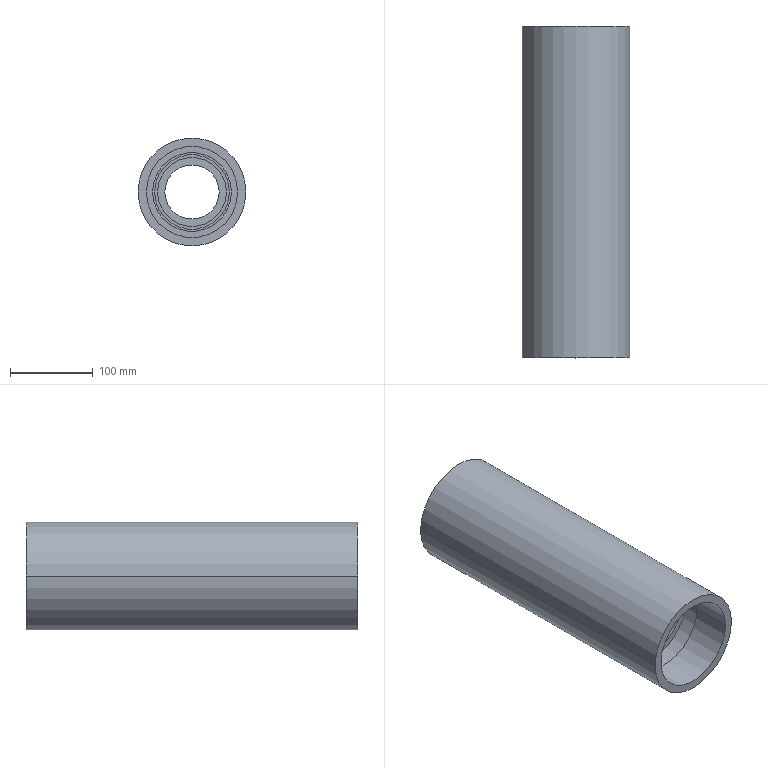Part | SolidWorks | features BaseBody 1 | 1 solid | 36 faces | box 130 x 400 x 130 mm | volume 2263150 mm3 | cylinder 24 | plane 12 | commonest cylinder face diameters 95 x6 110 x6 65.5 x2 76 x2 83 x2 90 x2
STEP:
#1=CARTESIAN_POINT('',(-2197.95,1104.894,-1577.624));
#2=VERTEX_POINT('',#1);
#3=CARTESIAN_POINT('',(-2197.95,704.894,-1577.624));
#4=VERTEX_POINT('',#3);
#5=CARTESIAN_POINT('',(-2197.95,1104.894,-1577.624));
#6=DIRECTION('',(0.,-1.,0.));
#7=VECTOR('',#6,1000.);
#8=LINE('',#5,#7);
#9=EDGE_CURVE('',#2,#4,#8,.T.);
#10=ORIENTED_EDGE('',*,*,#9,.F.);
#11=CARTESIAN_POINT('',(-2067.95,1104.894,-1577.624));
#12=VERTEX_POINT('',#11);
#13=CARTESIAN_POINT('',(-2132.95,1104.894,-1577.624));
#14=DIRECTION('',(0.,1.,0.));
#15=DIRECTION('',(1.,0.,0.));
#16=AXIS2_PLACEMENT_3D('',#13,#14,#15);
#17=CIRCLE('',#16,65.);
#18=EDGE_CURVE('',#12,#2,#17,.T.);
#19=ORIENTED_EDGE('',*,*,#18,.F.);
#20=CARTESIAN_POINT('',(-2067.95,704.894,-1577.624));
#21=VERTEX_POINT('',#20);
#22=CARTESIAN_POINT('',(-2067.95,1104.894,-1577.624));
#23=DIRECTION('',(0.,-1.,0.));
#24=VECTOR('',#23,1000.);
#25=LINE('',#22,#24);
#26=EDGE_CURVE('',#12,#21,#25,.T.);
#27=ORIENTED_EDGE('',*,*,#26,.T.);
#28=CARTESIAN_POINT('',(-2132.95,704.894,-1577.624));
#29=DIRECTION('',(0.,-1.,0.));
#30=DIRECTION('',(-1.,0.,0.));
#31=AXIS2_PLACEMENT_3D('',#28,#29,#30);
#32=CIRCLE('',#31,65.);
#33=EDGE_CURVE('',#4,#21,#32,.T.);
#34=ORIENTED_EDGE('',*,*,#33,.F.);
#35=EDGE_LOOP('',(#10,#19,#27,#34));
#36=FACE_OUTER_BOUND('',#35,.T.);
#37=CARTESIAN_POINT('',(-2132.95,1104.894,-1577.624));
#38=DIRECTION('',(0.,1.,0.));
#39=DIRECTION('',(1.,0.,0.));
#40=AXIS2_PLACEMENT_3D('',#37,#38,#39);
#41=CYLINDRICAL_SURFACE('',#40,65.);
#42=ADVANCED_FACE('',(#36),#41,.T.);
#43=CARTESIAN_POINT('',(-2077.95,704.894,-1577.624));
#44=VERTEX_POINT('',#43);
#45=CARTESIAN_POINT('',(-2187.95,704.894,-1577.624));
#46=VERTEX_POINT('',#45);
#47=CARTESIAN_POINT('',(-2132.95,704.894,-1577.624));
#48=DIRECTION('',(0.,-1.,0.));
#49=DIRECTION('',(1.,0.,0.));
#50=AXIS2_PLACEMENT_3D('',#47,#48,#49);
#51=CIRCLE('',#50,55.);
#52=EDGE_CURVE('',#44,#46,#51,.T.);
#53=ORIENTED_EDGE('',*,*,#52,.F.);
#54=CARTESIAN_POINT('',(-2132.95,704.894,-1577.624));
#55=DIRECTION('',(0.,-1.,0.));
#56=DIRECTION('',(-1.,0.,0.));
#57=AXIS2_PLACEMENT_3D('',#54,#55,#56);
#58=CIRCLE('',#57,55.);
#59=EDGE_CURVE('',#46,#44,#58,.T.);
#60=ORIENTED_EDGE('',*,*,#59,.F.);
#61=EDGE_LOOP('',(#53,#60));
#62=FACE_BOUND('',#61,.T.);
#63=ORIENTED_EDGE('',*,*,#33,.T.);
#64=CARTESIAN_POINT('',(-2132.95,704.894,-1577.624));
#65=DIRECTION('',(0.,-1.,0.));
#66=DIRECTION('',(1.,0.,0.));
#67=AXIS2_PLACEMENT_3D('',#64,#65,#66);
#68=CIRCLE('',#67,65.);
#69=EDGE_CURVE('',#21,#4,#68,.T.);
#70=ORIENTED_EDGE('',*,*,#69,.T.);
#71=EDGE_LOOP('',(#63,#70));
#72=FACE_OUTER_BOUND('',#71,.T.);
#73=CARTESIAN_POINT('',(-2066.65,704.894,-1643.924));
#74=DIRECTION('',(0.,-1.,0.));
#75=DIRECTION('',(0.,0.,-1.));
#76=AXIS2_PLACEMENT_3D('',#73,#74,#75);
#77=PLANE('',#76);
#78=ADVANCED_FACE('',(#62,#72),#77,.T.);
#79=CARTESIAN_POINT('',(-2132.95,1104.894,-1577.624));
#80=DIRECTION('',(0.,1.,0.));
#81=DIRECTION('',(-1.,0.,0.));
#82=AXIS2_PLACEMENT_3D('',#79,#80,#81);
#83=CIRCLE('',#82,65.);
#84=EDGE_CURVE('',#2,#12,#83,.T.);
#85=ORIENTED_EDGE('',*,*,#84,.F.);
#86=ORIENTED_EDGE('',*,*,#9,.T.);
#87=ORIENTED_EDGE('',*,*,#69,.F.);
#88=ORIENTED_EDGE('',*,*,#26,.F.);
#89=EDGE_LOOP('',(#85,#86,#87,#88));
#90=FACE_OUTER_BOUND('',#89,.T.);
#91=CARTESIAN_POINT('',(-2132.95,1104.894,-1577.624));
#92=DIRECTION('',(0.,1.,0.));
#93=DIRECTION('',(-1.,0.,0.));
#94=AXIS2_PLACEMENT_3D('',#91,#92,#93);
#95=CYLINDRICAL_SURFACE('',#94,65.);
#96=ADVANCED_FACE('',(#90),#95,.T.);
#97=CARTESIAN_POINT('',(-2187.95,1104.894,-1577.624));
#98=VERTEX_POINT('',#97);
#99=CARTESIAN_POINT('',(-2077.95,1104.894,-1577.624));
#100=VERTEX_POINT('',#99);
#101=CARTESIAN_POINT('',(-2132.95,1104.894,-1577.624));
#102=DIRECTION('',(0.,1.,0.));
#103=DIRECTION('',(-1.,0.,0.));
#104=AXIS2_PLACEMENT_3D('',#101,#102,#103);
#105=CIRCLE('',#104,55.);
#106=EDGE_CURVE('',#98,#100,#105,.T.);
#107=ORIENTED_EDGE('',*,*,#106,.F.);
#108=CARTESIAN_POINT('',(-2132.95,1104.894,-1577.624));
#109=DIRECTION('',(0.,1.,0.));
#110=DIRECTION('',(1.,0.,0.));
#111=AXIS2_PLACEMENT_3D('',#108,#109,#110);
#112=CIRCLE('',#111,55.);
#113=EDGE_CURVE('',#100,#98,#112,.T.);
#114=ORIENTED_EDGE('',*,*,#113,.F.);
#115=EDGE_LOOP('',(#107,#114));
#116=FACE_BOUND('',#115,.T.);
#117=ORIENTED_EDGE('',*,*,#18,.T.);
#118=ORIENTED_EDGE('',*,*,#84,.T.);
#119=EDGE_LOOP('',(#117,#118));
#120=FACE_OUTER_BOUND('',#119,.T.);
#121=CARTESIAN_POINT('',(-2066.65,1104.894,-1511.324));
#122=DIRECTION('',(0.,1.,0.));
#123=DIRECTION('',(1.,0.,0.));
#124=AXIS2_PLACEMENT_3D('',#121,#122,#123);
#125=PLANE('',#124);
#126=ADVANCED_FACE('',(#116,#120),#125,.T.);
#127=CARTESIAN_POINT('',(-2187.95,753.694,-1577.624));
#128=VERTEX_POINT('',#127);
#129=CARTESIAN_POINT('',(-2077.95,753.694,-1577.624));
#130=VERTEX_POINT('',#129);
#131=CARTESIAN_POINT('',(-2132.95,753.694,-1577.624));
#132=DIRECTION('',(0.,-1.,0.));
#133=DIRECTION('',(-1.,0.,0.));
#134=AXIS2_PLACEMENT_3D('',#131,#132,#133);
#135=CIRCLE('',#134,55.);
#136=EDGE_CURVE('',#128,#130,#135,.T.);
#137=ORIENTED_EDGE('',*,*,#136,.F.);
#138=CARTESIAN_POINT('',(-2187.95,753.694,-1577.624));
#139=DIRECTION('',(0.,-1.,0.));
#140=VECTOR('',#139,1000.);
#141=LINE('',#138,#140);
#142=EDGE_CURVE('',#128,#46,#141,.T.);
#143=ORIENTED_EDGE('',*,*,#142,.T.);
#144=ORIENTED_EDGE('',*,*,#59,.T.);
#145=CARTESIAN_POINT('',(-2077.95,753.694,-1577.624));
#146=DIRECTION('',(0.,-1.,0.));
#147=VECTOR('',#146,1000.);
#148=LINE('',#145,#147);
#149=EDGE_CURVE('',#130,#44,#148,.T.);
#150=ORIENTED_EDGE('',*,*,#149,.F.);
#151=EDGE_LOOP('',(#137,#143,#144,#150));
#152=FACE_OUTER_BOUND('',#151,.T.);
#153=CARTESIAN_POINT('',(-2132.95,753.894,-1577.624));
#154=DIRECTION('',(0.,1.,0.));
#155=DIRECTION('',(1.,0.,0.));
#156=AXIS2_PLACEMENT_3D('',#153,#154,#155);
#157=CYLINDRICAL_SURFACE('',#156,55.);
#158=ADVANCED_FACE('',(#152),#157,.F.);
#159=ORIENTED_EDGE('',*,*,#52,.T.);
#160=ORIENTED_EDGE('',*,*,#142,.F.);
#161=CARTESIAN_POINT('',(-2132.95,753.694,-1577.624));
#162=DIRECTION('',(0.,-1.,0.));
#163=DIRECTION('',(1.,0.,0.));
#164=AXIS2_PLACEMENT_3D('',#161,#162,#163);
#165=CIRCLE('',#164,55.);
#166=EDGE_CURVE('',#130,#128,#165,.T.);
#167=ORIENTED_EDGE('',*,*,#166,.F.);
#168=ORIENTED_EDGE('',*,*,#149,.T.);
#169=EDGE_LOOP('',(#159,#160,#167,#168));
#170=FACE_OUTER_BOUND('',#169,.T.);
#171=CARTESIAN_POINT('',(-2132.95,753.894,-1577.624));
#172=DIRECTION('',(0.,1.,0.));
#173=DIRECTION('',(-1.,0.,0.));
#174=AXIS2_PLACEMENT_3D('',#171,#172,#173);
#175=CYLINDRICAL_SURFACE('',#174,55.);
#176=ADVANCED_FACE('',(#170),#175,.F.);
#177=CARTESIAN_POINT('',(-2070.45,778.694,-1577.624));
#178=VERTEX_POINT('',#177);
#179=CARTESIAN_POINT('',(-2070.45,753.694,-1577.624));
#180=VERTEX_POINT('',#179);
#181=CARTESIAN_POINT('',(-2070.45,778.694,-1577.624));
#182=DIRECTION('',(0.,-1.,0.));
#183=VECTOR('',#182,1000.);
#184=LINE('',#181,#183);
#185=EDGE_CURVE('',#178,#180,#184,.T.);
#186=ORIENTED_EDGE('',*,*,#185,.F.);
#187=CARTESIAN_POINT('',(-2195.45,778.694,-1577.624));
#188=VERTEX_POINT('',#187);
#189=CARTESIAN_POINT('',(-2132.95,778.694,-1577.624));
#190=DIRECTION('',(0.,1.,0.));
#191=DIRECTION('',(1.,0.,0.));
#192=AXIS2_PLACEMENT_3D('',#189,#190,#191);
#193=CIRCLE('',#192,62.5);
#194=EDGE_CURVE('',#178,#188,#193,.T.);
#195=ORIENTED_EDGE('',*,*,#194,.T.);
#196=CARTESIAN_POINT('',(-2195.45,753.694,-1577.624));
#197=VERTEX_POINT('',#196);
#198=CARTESIAN_POINT('',(-2195.45,778.694,-1577.624));
#199=DIRECTION('',(0.,-1.,0.));
#200=VECTOR('',#199,1000.);
#201=LINE('',#198,#200);
#202=EDGE_CURVE('',#188,#197,#201,.T.);
#203=ORIENTED_EDGE('',*,*,#202,.T.);
#204=CARTESIAN_POINT('',(-2132.95,753.694,-1577.624));
#205=DIRECTION('',(0.,-1.,0.));
#206=DIRECTION('',(-1.,0.,0.));
#207=AXIS2_PLACEMENT_3D('',#204,#205,#206);
#208=CIRCLE('',#207,62.5);
#209=EDGE_CURVE('',#197,#180,#208,.T.);
#210=ORIENTED_EDGE('',*,*,#209,.T.);
#211=EDGE_LOOP('',(#186,#195,#203,#210));
#212=FACE_OUTER_BOUND('',#211,.T.);
#213=CARTESIAN_POINT('',(-2132.95,778.694,-1577.624));
#214=DIRECTION('',(0.,1.,0.));
#215=DIRECTION('',(1.,0.,0.));
#216=AXIS2_PLACEMENT_3D('',#213,#214,#215);
#217=CYLINDRICAL_SURFACE('',#216,62.5);
#218=ADVANCED_FACE('',(#212),#217,.F.);
#219=ORIENTED_EDGE('',*,*,#166,.T.);
#220=ORIENTED_EDGE('',*,*,#136,.T.);
#221=EDGE_LOOP('',(#219,#220));
#222=FACE_BOUND('',#221,.T.);
#223=ORIENTED_EDGE('',*,*,#209,.F.);
#224=CARTESIAN_POINT('',(-2132.95,753.694,-1577.624));
#225=DIRECTION('',(0.,-1.,0.));
#226=DIRECTION('',(1.,0.,0.));
#227=AXIS2_PLACEMENT_3D('',#224,#225,#226);
#228=CIRCLE('',#227,62.5);
#229=EDGE_CURVE('',#180,#197,#228,.T.);
#230=ORIENTED_EDGE('',*,*,#229,.F.);
#231=EDGE_LOOP('',(#223,#230));
#232=FACE_OUTER_BOUND('',#231,.T.);
#233=CARTESIAN_POINT('',(-2069.2,753.694,-1641.374));
#234=DIRECTION('',(0.,1.,0.));
#235=DIRECTION('',(1.,0.,0.));
#236=AXIS2_PLACEMENT_3D('',#233,#234,#235);
#237=PLANE('',#236);
#238=ADVANCED_FACE('',(#222,#232),#237,.T.);
#239=ORIENTED_EDGE('',*,*,#229,.T.);
#240=ORIENTED_EDGE('',*,*,#202,.F.);
#241=CARTESIAN_POINT('',(-2132.95,778.694,-1577.624));
#242=DIRECTION('',(0.,1.,0.));
#243=DIRECTION('',(-1.,0.,0.));
#244=AXIS2_PLACEMENT_3D('',#241,#242,#243);
#245=CIRCLE('',#244,62.5);
#246=EDGE_CURVE('',#188,#178,#245,.T.);
#247=ORIENTED_EDGE('',*,*,#246,.T.);
#248=ORIENTED_EDGE('',*,*,#185,.T.);
#249=EDGE_LOOP('',(#239,#240,#247,#248));
#250=FACE_OUTER_BOUND('',#249,.T.);
#251=CARTESIAN_POINT('',(-2132.95,778.694,-1577.624));
#252=DIRECTION('',(0.,1.,0.));
#253=DIRECTION('',(-1.,0.,0.));
#254=AXIS2_PLACEMENT_3D('',#251,#252,#253);
#255=CYLINDRICAL_SURFACE('',#254,62.5);
#256=ADVANCED_FACE('',(#250),#255,.F.);
#257=CARTESIAN_POINT('',(-2187.95,778.694,-1577.624));
#258=VERTEX_POINT('',#257);
#259=CARTESIAN_POINT('',(-2077.95,778.694,-1577.624));
#260=VERTEX_POINT('',#259);
#261=CARTESIAN_POINT('',(-2132.95,778.694,-1577.624));
#262=DIRECTION('',(0.,1.,0.));
#263=DIRECTION('',(-1.,0.,0.));
#264=AXIS2_PLACEMENT_3D('',#261,#262,#263);
#265=CIRCLE('',#264,55.);
#266=EDGE_CURVE('',#258,#260,#265,.T.);
#267=ORIENTED_EDGE('',*,*,#266,.T.);
#268=CARTESIAN_POINT('',(-2132.95,778.694,-1577.624));
#269=DIRECTION('',(0.,1.,0.));
#270=DIRECTION('',(1.,0.,0.));
#271=AXIS2_PLACEMENT_3D('',#268,#269,#270);
#272=CIRCLE('',#271,55.);
#273=EDGE_CURVE('',#260,#258,#272,.T.);
#274=ORIENTED_EDGE('',*,*,#273,.T.);
#275=EDGE_LOOP('',(#267,#274));
#276=FACE_BOUND('',#275,.T.);
#277=ORIENTED_EDGE('',*,*,#194,.F.);
#278=ORIENTED_EDGE('',*,*,#246,.F.);
#279=EDGE_LOOP('',(#277,#278));
#280=FACE_OUTER_BOUND('',#279,.T.);
#281=CARTESIAN_POINT('',(-2069.2,778.694,-1513.874));
#282=DIRECTION('',(0.,-1.,0.));
#283=DIRECTION('',(0.,0.,-1.));
#284=AXIS2_PLACEMENT_3D('',#281,#282,#283);
#285=PLANE('',#284);
#286=ADVANCED_FACE('',(#276,#280),#285,.T.);
#287=CARTESIAN_POINT('',(-2077.95,813.694,-1577.624));
#288=VERTEX_POINT('',#287);
#289=CARTESIAN_POINT('',(-2187.95,813.694,-1577.624));
#290=VERTEX_POINT('',#289);
#291=CARTESIAN_POINT('',(-2132.95,813.694,-1577.624));
#292=DIRECTION('',(0.,1.,0.));
#293=DIRECTION('',(1.,0.,0.));
#294=AXIS2_PLACEMENT_3D('',#291,#292,#293);
#295=CIRCLE('',#294,55.);
#296=EDGE_CURVE('',#288,#290,#295,.T.);
#297=ORIENTED_EDGE('',*,*,#296,.T.);
#298=CARTESIAN_POINT('',(-2187.95,813.694,-1577.624));
#299=DIRECTION('',(0.,-1.,0.));
#300=VECTOR('',#299,1000.);
#301=LINE('',#298,#300);
#302=EDGE_CURVE('',#290,#258,#301,.T.);
#303=ORIENTED_EDGE('',*,*,#302,.T.);
#304=ORIENTED_EDGE('',*,*,#273,.F.);
#305=CARTESIAN_POINT('',(-2077.95,813.694,-1577.624));
#306=DIRECTION('',(0.,-1.,0.));
#307=VECTOR('',#306,1000.);
#308=LINE('',#305,#307);
#309=EDGE_CURVE('',#288,#260,#308,.T.);
#310=ORIENTED_EDGE('',*,*,#309,.F.);
#311=EDGE_LOOP('',(#297,#303,#304,#310));
#312=FACE_OUTER_BOUND('',#311,.T.);
#313=CARTESIAN_POINT('',(-2132.95,813.694,-1577.624));
#314=DIRECTION('',(0.,1.,0.));
#315=DIRECTION('',(1.,0.,0.));
#316=AXIS2_PLACEMENT_3D('',#313,#314,#315);
#317=CYLINDRICAL_SURFACE('',#316,55.);
#318=ADVANCED_FACE('',(#312),#317,.F.);
#319=ORIENTED_EDGE('',*,*,#266,.F.);
#320=ORIENTED_EDGE('',*,*,#302,.F.);
#321=CARTESIAN_POINT('',(-2132.95,813.694,-1577.624));
#322=DIRECTION('',(0.,1.,0.));
#323=DIRECTION('',(-1.,0.,0.));
#324=AXIS2_PLACEMENT_3D('',#321,#322,#323);
#325=CIRCLE('',#324,55.);
#326=EDGE_CURVE('',#290,#288,#325,.T.);
#327=ORIENTED_EDGE('',*,*,#326,.T.);
#328=ORIENTED_EDGE('',*,*,#309,.T.);
#329=EDGE_LOOP('',(#319,#320,#327,#328));
#330=FACE_OUTER_BOUND('',#329,.T.);
#331=CARTESIAN_POINT('',(-2132.95,813.694,-1577.624));
#332=DIRECTION('',(0.,1.,0.));
#333=DIRECTION('',(-1.,0.,0.));
#334=AXIS2_PLACEMENT_3D('',#331,#332,#333);
#335=CYLINDRICAL_SURFACE('',#334,55.);
#336=ADVANCED_FACE('',(#330),#335,.F.);
#337=CARTESIAN_POINT('',(-2180.45,813.694,-1577.624));
#338=VERTEX_POINT('',#337);
#339=CARTESIAN_POINT('',(-2085.45,813.694,-1577.624));
#340=VERTEX_POINT('',#339);
#341=CARTESIAN_POINT('',(-2132.95,813.694,-1577.624));
#342=DIRECTION('',(0.,1.,0.));
#343=DIRECTION('',(-1.,0.,0.));
#344=AXIS2_PLACEMENT_3D('',#341,#342,#343);
#345=CIRCLE('',#344,47.5);
#346=EDGE_CURVE('',#338,#340,#345,.T.);
#347=ORIENTED_EDGE('',*,*,#346,.T.);
#348=CARTESIAN_POINT('',(-2132.95,813.694,-1577.624));
#349=DIRECTION('',(0.,1.,0.));
#350=DIRECTION('',(1.,0.,0.));
#351=AXIS2_PLACEMENT_3D('',#348,#349,#350);
#352=CIRCLE('',#351,47.5);
#353=EDGE_CURVE('',#340,#338,#352,.T.);
#354=ORIENTED_EDGE('',*,*,#353,.T.);
#355=EDGE_LOOP('',(#347,#354));
#356=FACE_BOUND('',#355,.T.);
#357=ORIENTED_EDGE('',*,*,#296,.F.);
#358=ORIENTED_EDGE('',*,*,#326,.F.);
#359=EDGE_LOOP('',(#357,#358));
#360=FACE_OUTER_BOUND('',#359,.T.);
#361=CARTESIAN_POINT('',(-2076.85,813.694,-1521.524));
#362=DIRECTION('',(0.,-1.,0.));
#363=DIRECTION('',(0.,0.,-1.));
#364=AXIS2_PLACEMENT_3D('',#361,#362,#363);
#365=PLANE('',#364);
#366=ADVANCED_FACE('',(#356,#360),#365,.T.);
#367=CARTESIAN_POINT('',(-2180.45,825.094,-1577.624));
#368=VERTEX_POINT('',#367);
#369=CARTESIAN_POINT('',(-2085.45,825.094,-1577.624));
#370=VERTEX_POINT('',#369);
#371=CARTESIAN_POINT('',(-2132.95,825.094,-1577.624));
#372=DIRECTION('',(0.,1.,0.));
#373=DIRECTION('',(-1.,0.,0.));
#374=AXIS2_PLACEMENT_3D('',#371,#372,#373);
#375=CIRCLE('',#374,47.5);
#376=EDGE_CURVE('',#368,#370,#375,.T.);
#377=ORIENTED_EDGE('',*,*,#376,.F.);
#378=CARTESIAN_POINT('',(-2180.45,927.094,-1577.624));
#379=VERTEX_POINT('',#378);
#380=CARTESIAN_POINT('',(-2180.45,927.094,-1577.624));
#381=DIRECTION('',(0.,-1.,0.));
#382=VECTOR('',#381,1000.);
#383=LINE('',#380,#382);
#384=EDGE_CURVE('',#379,#368,#383,.T.);
#385=ORIENTED_EDGE('',*,*,#384,.F.);
#386=CARTESIAN_POINT('',(-2085.45,927.094,-1577.624));
#387=VERTEX_POINT('',#386);
#388=CARTESIAN_POINT('',(-2132.95,927.094,-1577.624));
#389=DIRECTION('',(0.,1.,0.));
#390=DIRECTION('',(-1.,0.,0.));
#391=AXIS2_PLACEMENT_3D('',#388,#389,#390);
#392=CIRCLE('',#391,47.5);
#393=EDGE_CURVE('',#379,#387,#392,.T.);
#394=ORIENTED_EDGE('',*,*,#393,.T.);
#395=CARTESIAN_POINT('',(-2085.45,927.094,-1577.624));
#396=DIRECTION('',(0.,-1.,0.));
#397=VECTOR('',#396,1000.);
#398=LINE('',#395,#397);
#399=EDGE_CURVE('',#387,#370,#398,.T.);
#400=ORIENTED_EDGE('',*,*,#399,.T.);
#401=EDGE_LOOP('',(#377,#385,#394,#400));
#402=FACE_OUTER_BOUND('',#401,.T.);
#403=CARTESIAN_POINT('',(-2132.95,927.094,-1577.624));
#404=DIRECTION('',(0.,1.,0.));
#405=DIRECTION('',(-1.,0.,0.));
#406=AXIS2_PLACEMENT_3D('',#403,#404,#405);
#407=CYLINDRICAL_SURFACE('',#406,47.5);
#408=ADVANCED_FACE('',(#402),#407,.F.);
#409=CARTESIAN_POINT('',(-2132.95,927.094,-1577.624));
#410=DIRECTION('',(0.,1.,0.));
#411=DIRECTION('',(1.,0.,0.));
#412=AXIS2_PLACEMENT_3D('',#409,#410,#411);
#413=CIRCLE('',#412,47.5);
#414=EDGE_CURVE('',#387,#379,#413,.T.);
#415=ORIENTED_EDGE('',*,*,#414,.T.);
#416=ORIENTED_EDGE('',*,*,#384,.T.);
#417=CARTESIAN_POINT('',(-2132.95,825.094,-1577.624));
#418=DIRECTION('',(0.,1.,0.));
#419=DIRECTION('',(1.,0.,0.));
#420=AXIS2_PLACEMENT_3D('',#417,#418,#419);
#421=CIRCLE('',#420,47.5);
#422=EDGE_CURVE('',#370,#368,#421,.T.);
#423=ORIENTED_EDGE('',*,*,#422,.F.);
#424=ORIENTED_EDGE('',*,*,#399,.F.);
#425=EDGE_LOOP('',(#415,#416,#423,#424));
#426=FACE_OUTER_BOUND('',#425,.T.);
#427=CARTESIAN_POINT('',(-2132.95,927.094,-1577.624));
#428=DIRECTION('',(0.,1.,0.));
#429=DIRECTION('',(1.,0.,0.));
#430=AXIS2_PLACEMENT_3D('',#427,#428,#429);
#431=CYLINDRICAL_SURFACE('',#430,47.5);
#432=ADVANCED_FACE('',(#426),#431,.F.);
#433=CARTESIAN_POINT('',(-2085.45,815.094,-1577.624));
#434=VERTEX_POINT('',#433);
#435=CARTESIAN_POINT('',(-2085.45,815.094,-1577.624));
#436=DIRECTION('',(0.,-1.,0.));
#437=VECTOR('',#436,1000.);
#438=LINE('',#435,#437);
#439=EDGE_CURVE('',#434,#340,#438,.T.);
#440=ORIENTED_EDGE('',*,*,#439,.F.);
#441=CARTESIAN_POINT('',(-2180.45,815.094,-1577.624));
#442=VERTEX_POINT('',#441);
#443=CARTESIAN_POINT('',(-2132.95,815.094,-1577.624));
#444=DIRECTION('',(0.,-1.,0.));
#445=DIRECTION('',(-1.,0.,0.));
#446=AXIS2_PLACEMENT_3D('',#443,#444,#445);
#447=CIRCLE('',#446,47.5);
#448=EDGE_CURVE('',#442,#434,#447,.T.);
#449=ORIENTED_EDGE('',*,*,#448,.F.);
#450=CARTESIAN_POINT('',(-2180.45,815.094,-1577.624));
#451=DIRECTION('',(0.,-1.,0.));
#452=VECTOR('',#451,1000.);
#453=LINE('',#450,#452);
#454=EDGE_CURVE('',#442,#338,#453,.T.);
#455=ORIENTED_EDGE('',*,*,#454,.T.);
#456=ORIENTED_EDGE('',*,*,#353,.F.);
#457=EDGE_LOOP('',(#440,#449,#455,#456));
#458=FACE_OUTER_BOUND('',#457,.T.);
#459=CARTESIAN_POINT('',(-2132.95,927.094,-1577.624));
#460=DIRECTION('',(0.,1.,0.));
#461=DIRECTION('',(1.,0.,0.));
#462=AXIS2_PLACEMENT_3D('',#459,#460,#461);
#463=CYLINDRICAL_SURFACE('',#462,47.5);
#464=ADVANCED_FACE('',(#458),#463,.F.);
#465=ORIENTED_EDGE('',*,*,#454,.F.);
#466=CARTESIAN_POINT('',(-2132.95,815.094,-1577.624));
#467=DIRECTION('',(0.,-1.,0.));
#468=DIRECTION('',(1.,0.,0.));
#469=AXIS2_PLACEMENT_3D('',#466,#467,#468);
#470=CIRCLE('',#469,47.5);
#471=EDGE_CURVE('',#434,#442,#470,.T.);
#472=ORIENTED_EDGE('',*,*,#471,.F.);
#473=ORIENTED_EDGE('',*,*,#439,.T.);
#474=ORIENTED_EDGE('',*,*,#346,.F.);
#475=EDGE_LOOP('',(#465,#472,#473,#474));
#476=FACE_OUTER_BOUND('',#475,.T.);
#477=CARTESIAN_POINT('',(-2132.95,927.094,-1577.624));
#478=DIRECTION('',(0.,1.,0.));
#479=DIRECTION('',(-1.,0.,0.));
#480=AXIS2_PLACEMENT_3D('',#477,#478,#479);
#481=CYLINDRICAL_SURFACE('',#480,47.5);
#482=ADVANCED_FACE('',(#476),#481,.F.);
#483=CARTESIAN_POINT('',(-2174.45,927.094,-1577.624));
#484=VERTEX_POINT('',#483);
#485=CARTESIAN_POINT('',(-2091.45,927.094,-1577.624));
#486=VERTEX_POINT('',#485);
#487=CARTESIAN_POINT('',(-2132.95,927.094,-1577.624));
#488=DIRECTION('',(0.,1.,0.));
#489=DIRECTION('',(-1.,0.,0.));
#490=AXIS2_PLACEMENT_3D('',#487,#488,#489);
#491=CIRCLE('',#490,41.5);
#492=EDGE_CURVE('',#484,#486,#491,.T.);
#493=ORIENTED_EDGE('',*,*,#492,.T.);
#494=CARTESIAN_POINT('',(-2132.95,927.094,-1577.624));
#495=DIRECTION('',(0.,1.,0.));
#496=DIRECTION('',(1.,0.,0.));
#497=AXIS2_PLACEMENT_3D('',#494,#495,#496);
#498=CIRCLE('',#497,41.5);
#499=EDGE_CURVE('',#486,#484,#498,.T.);
#500=ORIENTED_EDGE('',*,*,#499,.T.);
#501=EDGE_LOOP('',(#493,#500));
#502=FACE_BOUND('',#501,.T.);
#503=ORIENTED_EDGE('',*,*,#414,.F.);
#504=ORIENTED_EDGE('',*,*,#393,.F.);
#505=EDGE_LOOP('',(#503,#504));
#506=FACE_OUTER_BOUND('',#505,.T.);
#507=CARTESIAN_POINT('',(-2084.5,927.094,-1529.174));
#508=DIRECTION('',(0.,-1.,0.));
#509=DIRECTION('',(0.,0.,-1.));
#510=AXIS2_PLACEMENT_3D('',#507,#508,#509);
#511=PLANE('',#510);
#512=ADVANCED_FACE('',(#502,#506),#511,.T.);
#513=CARTESIAN_POINT('',(-2087.95,825.094,-1577.624));
#514=VERTEX_POINT('',#513);
#515=CARTESIAN_POINT('',(-2087.95,815.094,-1577.624));
#516=VERTEX_POINT('',#515);
#517=CARTESIAN_POINT('',(-2087.95,825.094,-1577.624));
#518=DIRECTION('',(0.,-1.,0.));
#519=VECTOR('',#518,1000.);
#520=LINE('',#517,#519);
#521=EDGE_CURVE('',#514,#516,#520,.T.);
#522=ORIENTED_EDGE('',*,*,#521,.F.);
#523=CARTESIAN_POINT('',(-2177.95,825.094,-1577.624));
#524=VERTEX_POINT('',#523);
#525=CARTESIAN_POINT('',(-2132.95,825.094,-1577.624));
#526=DIRECTION('',(0.,1.,0.));
#527=DIRECTION('',(1.,0.,0.));
#528=AXIS2_PLACEMENT_3D('',#525,#526,#527);
#529=CIRCLE('',#528,45.);
#530=EDGE_CURVE('',#514,#524,#529,.T.);
#531=ORIENTED_EDGE('',*,*,#530,.T.);
#532=CARTESIAN_POINT('',(-2177.95,815.094,-1577.624));
#533=VERTEX_POINT('',#532);
#534=CARTESIAN_POINT('',(-2177.95,825.094,-1577.624));
#535=DIRECTION('',(0.,-1.,0.));
#536=VECTOR('',#535,1000.);
#537=LINE('',#534,#536);
#538=EDGE_CURVE('',#524,#533,#537,.T.);
#539=ORIENTED_EDGE('',*,*,#538,.T.);
#540=CARTESIAN_POINT('',(-2132.95,815.094,-1577.624));
#541=DIRECTION('',(0.,-1.,0.));
#542=DIRECTION('',(-1.,0.,0.));
#543=AXIS2_PLACEMENT_3D('',#540,#541,#542);
#544=CIRCLE('',#543,45.);
#545=EDGE_CURVE('',#533,#516,#544,.T.);
#546=ORIENTED_EDGE('',*,*,#545,.T.);
#547=EDGE_LOOP('',(#522,#531,#539,#546));
#548=FACE_OUTER_BOUND('',#547,.T.);
#549=CARTESIAN_POINT('',(-2132.95,825.094,-1577.624));
#550=DIRECTION('',(0.,1.,0.));
#551=DIRECTION('',(1.,0.,0.));
#552=AXIS2_PLACEMENT_3D('',#549,#550,#551);
#553=CYLINDRICAL_SURFACE('',#552,45.);
#554=ADVANCED_FACE('',(#548),#553,.F.);
#555=ORIENTED_EDGE('',*,*,#545,.F.);
#556=CARTESIAN_POINT('',(-2132.95,815.094,-1577.624));
#557=DIRECTION('',(0.,-1.,0.));
#558=DIRECTION('',(1.,0.,0.));
#559=AXIS2_PLACEMENT_3D('',#556,#557,#558);
#560=CIRCLE('',#559,45.);
#561=EDGE_CURVE('',#516,#533,#560,.T.);
#562=ORIENTED_EDGE('',*,*,#561,.F.);
#563=EDGE_LOOP('',(#555,#562));
#564=FACE_BOUND('',#563,.T.);
#565=ORIENTED_EDGE('',*,*,#448,.T.);
#566=ORIENTED_EDGE('',*,*,#471,.T.);
#567=EDGE_LOOP('',(#565,#566));
#568=FACE_OUTER_BOUND('',#567,.T.);
#569=CARTESIAN_POINT('',(-2084.5,815.094,-1626.074));
#570=DIRECTION('',(0.,-1.,0.));
#571=DIRECTION('',(0.,0.,-1.));
#572=AXIS2_PLACEMENT_3D('',#569,#570,#571);
#573=PLANE('',#572);
#574=ADVANCED_FACE('',(#564,#568),#573,.T.);
#575=ORIENTED_EDGE('',*,*,#561,.T.);
#576=ORIENTED_EDGE('',*,*,#538,.F.);
#577=CARTESIAN_POINT('',(-2132.95,825.094,-1577.624));
#578=DIRECTION('',(0.,1.,0.));
#579=DIRECTION('',(-1.,0.,0.));
#580=AXIS2_PLACEMENT_3D('',#577,#578,#579);
#581=CIRCLE('',#580,45.);
#582=EDGE_CURVE('',#524,#514,#581,.T.);
#583=ORIENTED_EDGE('',*,*,#582,.T.);
#584=ORIENTED_EDGE('',*,*,#521,.T.);
#585=EDGE_LOOP('',(#575,#576,#583,#584));
#586=FACE_OUTER_BOUND('',#585,.T.);
#587=CARTESIAN_POINT('',(-2132.95,825.094,-1577.624));
#588=DIRECTION('',(0.,1.,0.));
#589=DIRECTION('',(-1.,0.,0.));
#590=AXIS2_PLACEMENT_3D('',#587,#588,#589);
#591=CYLINDRICAL_SURFACE('',#590,45.);
#592=ADVANCED_FACE('',(#586),#591,.F.);
#593=ORIENTED_EDGE('',*,*,#530,.F.);
#594=ORIENTED_EDGE('',*,*,#582,.F.);
#595=EDGE_LOOP('',(#593,#594));
#596=FACE_BOUND('',#595,.T.);
#597=ORIENTED_EDGE('',*,*,#422,.T.);
#598=ORIENTED_EDGE('',*,*,#376,.T.);
#599=EDGE_LOOP('',(#597,#598));
#600=FACE_OUTER_BOUND('',#599,.T.);
#601=CARTESIAN_POINT('',(-2084.5,825.094,-1529.174));
#602=DIRECTION('',(0.,1.,0.));
#603=DIRECTION('',(1.,0.,0.));
#604=AXIS2_PLACEMENT_3D('',#601,#602,#603);
#605=PLANE('',#604);
#606=ADVANCED_FACE('',(#596,#600),#605,.T.);
#607=CARTESIAN_POINT('',(-2077.95,1022.004,-1577.624));
#608=VERTEX_POINT('',#607);
#609=CARTESIAN_POINT('',(-2077.95,1104.894,-1577.624));
#610=DIRECTION('',(0.,-1.,0.));
#611=VECTOR('',#610,1000.);
#612=LINE('',#609,#611);
#613=EDGE_CURVE('',#100,#608,#612,.T.);
#614=ORIENTED_EDGE('',*,*,#613,.F.);
#615=ORIENTED_EDGE('',*,*,#113,.T.);
#616=CARTESIAN_POINT('',(-2187.95,1022.004,-1577.624));
#617=VERTEX_POINT('',#616);
#618=CARTESIAN_POINT('',(-2187.95,1104.894,-1577.624));
#619=DIRECTION('',(0.,-1.,0.));
#620=VECTOR('',#619,1000.);
#621=LINE('',#618,#620);
#622=EDGE_CURVE('',#98,#617,#621,.T.);
#623=ORIENTED_EDGE('',*,*,#622,.T.);
#624=CARTESIAN_POINT('',(-2132.95,1022.004,-1577.624));
#625=DIRECTION('',(0.,-1.,0.));
#626=DIRECTION('',(-1.,0.,0.));
#627=AXIS2_PLACEMENT_3D('',#624,#625,#626);
#628=CIRCLE('',#627,55.);
#629=EDGE_CURVE('',#617,#608,#628,.T.);
#630=ORIENTED_EDGE('',*,*,#629,.T.);
#631=EDGE_LOOP('',(#614,#615,#623,#630));
#632=FACE_OUTER_BOUND('',#631,.T.);
#633=CARTESIAN_POINT('',(-2132.95,1422.004,-1577.624));
#634=DIRECTION('',(0.,1.,0.));
#635=DIRECTION('',(1.,0.,0.));
#636=AXIS2_PLACEMENT_3D('',#633,#634,#635);
#637=CYLINDRICAL_SURFACE('',#636,55.);
#638=ADVANCED_FACE('',(#632),#637,.F.);
#639=CARTESIAN_POINT('',(-2085.45,1022.004,-1577.624));
#640=VERTEX_POINT('',#639);
#641=CARTESIAN_POINT('',(-2180.45,1022.004,-1577.624));
#642=VERTEX_POINT('',#641);
#643=CARTESIAN_POINT('',(-2132.95,1022.004,-1577.624));
#644=DIRECTION('',(0.,-1.,0.));
#645=DIRECTION('',(1.,0.,0.));
#646=AXIS2_PLACEMENT_3D('',#643,#644,#645);
#647=CIRCLE('',#646,47.5);
#648=EDGE_CURVE('',#640,#642,#647,.T.);
#649=ORIENTED_EDGE('',*,*,#648,.T.);
#650=CARTESIAN_POINT('',(-2132.95,1022.004,-1577.624));
#651=DIRECTION('',(0.,-1.,0.));
#652=DIRECTION('',(-1.,0.,0.));
#653=AXIS2_PLACEMENT_3D('',#650,#651,#652);
#654=CIRCLE('',#653,47.5);
#655=EDGE_CURVE('',#642,#640,#654,.T.);
#656=ORIENTED_EDGE('',*,*,#655,.T.);
#657=EDGE_LOOP('',(#649,#656));
#658=FACE_BOUND('',#657,.T.);
#659=ORIENTED_EDGE('',*,*,#629,.F.);
#660=CARTESIAN_POINT('',(-2132.95,1022.004,-1577.624));
#661=DIRECTION('',(0.,-1.,0.));
#662=DIRECTION('',(1.,0.,0.));
#663=AXIS2_PLACEMENT_3D('',#660,#661,#662);
#664=CIRCLE('',#663,55.);
#665=EDGE_CURVE('',#608,#617,#664,.T.);
#666=ORIENTED_EDGE('',*,*,#665,.F.);
#667=EDGE_LOOP('',(#659,#666));
#668=FACE_OUTER_BOUND('',#667,.T.);
#669=CARTESIAN_POINT('',(-2076.85,1022.004,-1633.724));
#670=DIRECTION('',(0.,1.,0.));
#671=DIRECTION('',(1.,0.,0.));
#672=AXIS2_PLACEMENT_3D('',#669,#670,#671);
#673=PLANE('',#672);
#674=ADVANCED_FACE('',(#658,#668),#673,.T.);
#675=ORIENTED_EDGE('',*,*,#665,.T.);
#676=ORIENTED_EDGE('',*,*,#622,.F.);
#677=ORIENTED_EDGE('',*,*,#106,.T.);
#678=ORIENTED_EDGE('',*,*,#613,.T.);
#679=EDGE_LOOP('',(#675,#676,#677,#678));
#680=FACE_OUTER_BOUND('',#679,.T.);
#681=CARTESIAN_POINT('',(-2132.95,1422.004,-1577.624));
#682=DIRECTION('',(0.,1.,0.));
#683=DIRECTION('',(-1.,0.,0.));
#684=AXIS2_PLACEMENT_3D('',#681,#682,#683);
#685=CYLINDRICAL_SURFACE('',#684,55.);
#686=ADVANCED_FACE('',(#680),#685,.F.);
#687=CARTESIAN_POINT('',(-2094.95,1018.004,-1577.624));
#688=VERTEX_POINT('',#687);
#689=CARTESIAN_POINT('',(-2094.95,1013.004,-1577.624));
#690=VERTEX_POINT('',#689);
#691=CARTESIAN_POINT('',(-2094.95,1018.004,-1577.624));
#692=DIRECTION('',(0.,-1.,0.));
#693=VECTOR('',#692,1000.);
#694=LINE('',#691,#693);
#695=EDGE_CURVE('',#688,#690,#694,.T.);
#696=ORIENTED_EDGE('',*,*,#695,.F.);
#697=CARTESIAN_POINT('',(-2170.95,1018.004,-1577.624));
#698=VERTEX_POINT('',#697);
#699=CARTESIAN_POINT('',(-2132.95,1018.004,-1577.624));
#700=DIRECTION('',(0.,-1.,0.));
#701=DIRECTION('',(-1.,0.,0.));
#702=AXIS2_PLACEMENT_3D('',#699,#700,#701);
#703=CIRCLE('',#702,38.);
#704=EDGE_CURVE('',#698,#688,#703,.T.);
#705=ORIENTED_EDGE('',*,*,#704,.F.);
#706=CARTESIAN_POINT('',(-2170.95,1013.004,-1577.624));
#707=VERTEX_POINT('',#706);
#708=CARTESIAN_POINT('',(-2170.95,1018.004,-1577.624));
#709=DIRECTION('',(0.,-1.,0.));
#710=VECTOR('',#709,1000.);
#711=LINE('',#708,#710);
#712=EDGE_CURVE('',#698,#707,#711,.T.);
#713=ORIENTED_EDGE('',*,*,#712,.T.);
#714=CARTESIAN_POINT('',(-2132.95,1013.004,-1577.624));
#715=DIRECTION('',(0.,-1.,0.));
#716=DIRECTION('',(-1.,0.,0.));
#717=AXIS2_PLACEMENT_3D('',#714,#715,#716);
#718=CIRCLE('',#717,38.);
#719=EDGE_CURVE('',#707,#690,#718,.T.);
#720=ORIENTED_EDGE('',*,*,#719,.T.);
#721=EDGE_LOOP('',(#696,#705,#713,#720));
#722=FACE_OUTER_BOUND('',#721,.T.);
#723=CARTESIAN_POINT('',(-2132.95,1413.004,-1577.624));
#724=DIRECTION('',(0.,1.,0.));
#725=DIRECTION('',(1.,0.,0.));
#726=AXIS2_PLACEMENT_3D('',#723,#724,#725);
#727=CYLINDRICAL_SURFACE('',#726,38.);
#728=ADVANCED_FACE('',(#722),#727,.F.);
#729=CARTESIAN_POINT('',(-2100.2,1013.004,-1577.624));
#730=VERTEX_POINT('',#729);
#731=CARTESIAN_POINT('',(-2165.7,1013.004,-1577.624));
#732=VERTEX_POINT('',#731);
#733=CARTESIAN_POINT('',(-2132.95,1013.004,-1577.624));
#734=DIRECTION('',(0.,-1.,0.));
#735=DIRECTION('',(1.,0.,0.));
#736=AXIS2_PLACEMENT_3D('',#733,#734,#735);
#737=CIRCLE('',#736,32.75);
#738=EDGE_CURVE('',#730,#732,#737,.T.);
#739=ORIENTED_EDGE('',*,*,#738,.T.);
#740=CARTESIAN_POINT('',(-2132.95,1013.004,-1577.624));
#741=DIRECTION('',(0.,-1.,0.));
#742=DIRECTION('',(-1.,0.,0.));
#743=AXIS2_PLACEMENT_3D('',#740,#741,#742);
#744=CIRCLE('',#743,32.75);
#745=EDGE_CURVE('',#732,#730,#744,.T.);
#746=ORIENTED_EDGE('',*,*,#745,.T.);
#747=EDGE_LOOP('',(#739,#746));
#748=FACE_BOUND('',#747,.T.);
#749=ORIENTED_EDGE('',*,*,#719,.F.);
#750=CARTESIAN_POINT('',(-2132.95,1013.004,-1577.624));
#751=DIRECTION('',(0.,-1.,0.));
#752=DIRECTION('',(1.,0.,0.));
#753=AXIS2_PLACEMENT_3D('',#750,#751,#752);
#754=CIRCLE('',#753,38.);
#755=EDGE_CURVE('',#690,#707,#754,.T.);
#756=ORIENTED_EDGE('',*,*,#755,.F.);
#757=EDGE_LOOP('',(#749,#756));
#758=FACE_OUTER_BOUND('',#757,.T.);
#759=CARTESIAN_POINT('',(-2094.19,1013.004,-1616.384));
#760=DIRECTION('',(0.,1.,0.));
#761=DIRECTION('',(1.,0.,0.));
#762=AXIS2_PLACEMENT_3D('',#759,#760,#761);
#763=PLANE('',#762);
#764=ADVANCED_FACE('',(#748,#758),#763,.T.);
#765=ORIENTED_EDGE('',*,*,#755,.T.);
#766=ORIENTED_EDGE('',*,*,#712,.F.);
#767=CARTESIAN_POINT('',(-2132.95,1018.004,-1577.624));
#768=DIRECTION('',(0.,-1.,0.));
#769=DIRECTION('',(1.,0.,0.));
#770=AXIS2_PLACEMENT_3D('',#767,#768,#769);
#771=CIRCLE('',#770,38.);
#772=EDGE_CURVE('',#688,#698,#771,.T.);
#773=ORIENTED_EDGE('',*,*,#772,.F.);
#774=ORIENTED_EDGE('',*,*,#695,.T.);
#775=EDGE_LOOP('',(#765,#766,#773,#774));
#776=FACE_OUTER_BOUND('',#775,.T.);
#777=CARTESIAN_POINT('',(-2132.95,1413.004,-1577.624));
#778=DIRECTION('',(0.,1.,0.));
#779=DIRECTION('',(-1.,0.,0.));
#780=AXIS2_PLACEMENT_3D('',#777,#778,#779);
#781=CYLINDRICAL_SURFACE('',#780,38.);
#782=ADVANCED_FACE('',(#776),#781,.F.);
#783=CARTESIAN_POINT('',(-2085.45,1018.004,-1577.624));
#784=VERTEX_POINT('',#783);
#785=CARTESIAN_POINT('',(-2085.45,1022.004,-1577.624));
#786=DIRECTION('',(0.,-1.,0.));
#787=VECTOR('',#786,1000.);
#788=LINE('',#785,#787);
#789=EDGE_CURVE('',#640,#784,#788,.T.);
#790=ORIENTED_EDGE('',*,*,#789,.F.);
#791=ORIENTED_EDGE('',*,*,#655,.F.);
#792=CARTESIAN_POINT('',(-2180.45,1018.004,-1577.624));
#793=VERTEX_POINT('',#792);
#794=CARTESIAN_POINT('',(-2180.45,1022.004,-1577.624));
#795=DIRECTION('',(0.,-1.,0.));
#796=VECTOR('',#795,1000.);
#797=LINE('',#794,#796);
#798=EDGE_CURVE('',#642,#793,#797,.T.);
#799=ORIENTED_EDGE('',*,*,#798,.T.);
#800=CARTESIAN_POINT('',(-2132.95,1018.004,-1577.624));
#801=DIRECTION('',(0.,-1.,0.));
#802=DIRECTION('',(-1.,0.,0.));
#803=AXIS2_PLACEMENT_3D('',#800,#801,#802);
#804=CIRCLE('',#803,47.5);
#805=EDGE_CURVE('',#793,#784,#804,.T.);
#806=ORIENTED_EDGE('',*,*,#805,.T.);
#807=EDGE_LOOP('',(#790,#791,#799,#806));
#808=FACE_OUTER_BOUND('',#807,.T.);
#809=CARTESIAN_POINT('',(-2132.95,1418.004,-1577.624));
#810=DIRECTION('',(0.,1.,0.));
#811=DIRECTION('',(1.,0.,0.));
#812=AXIS2_PLACEMENT_3D('',#809,#810,#811);
#813=CYLINDRICAL_SURFACE('',#812,47.5);
#814=ADVANCED_FACE('',(#808),#813,.F.);
#815=ORIENTED_EDGE('',*,*,#772,.T.);
#816=ORIENTED_EDGE('',*,*,#704,.T.);
#817=EDGE_LOOP('',(#815,#816));
#818=FACE_BOUND('',#817,.T.);
#819=ORIENTED_EDGE('',*,*,#805,.F.);
#820=CARTESIAN_POINT('',(-2132.95,1018.004,-1577.624));
#821=DIRECTION('',(0.,-1.,0.));
#822=DIRECTION('',(1.,0.,0.));
#823=AXIS2_PLACEMENT_3D('',#820,#821,#822);
#824=CIRCLE('',#823,47.5);
#825=EDGE_CURVE('',#784,#793,#824,.T.);
#826=ORIENTED_EDGE('',*,*,#825,.F.);
#827=EDGE_LOOP('',(#819,#826));
#828=FACE_OUTER_BOUND('',#827,.T.);
#829=CARTESIAN_POINT('',(-2084.5,1018.004,-1626.074));
#830=DIRECTION('',(0.,1.,0.));
#831=DIRECTION('',(1.,0.,0.));
#832=AXIS2_PLACEMENT_3D('',#829,#830,#831);
#833=PLANE('',#832);
#834=ADVANCED_FACE('',(#818,#828),#833,.T.);
#835=ORIENTED_EDGE('',*,*,#825,.T.);
#836=ORIENTED_EDGE('',*,*,#798,.F.);
#837=ORIENTED_EDGE('',*,*,#648,.F.);
#838=ORIENTED_EDGE('',*,*,#789,.T.);
#839=EDGE_LOOP('',(#835,#836,#837,#838));
#840=FACE_OUTER_BOUND('',#839,.T.);
#841=CARTESIAN_POINT('',(-2132.95,1418.004,-1577.624));
#842=DIRECTION('',(0.,1.,0.));
#843=DIRECTION('',(-1.,0.,0.));
#844=AXIS2_PLACEMENT_3D('',#841,#842,#843);
#845=CYLINDRICAL_SURFACE('',#844,47.5);
#846=ADVANCED_FACE('',(#840),#845,.F.);
#847=CARTESIAN_POINT('',(-2091.45,936.004,-1577.624));
#848=VERTEX_POINT('',#847);
#849=CARTESIAN_POINT('',(-2174.45,936.004,-1577.624));
#850=VERTEX_POINT('',#849);
#851=CARTESIAN_POINT('',(-2132.95,936.004,-1577.624));
#852=DIRECTION('',(0.,1.,0.));
#853=DIRECTION('',(1.,0.,0.));
#854=AXIS2_PLACEMENT_3D('',#851,#852,#853);
#855=CIRCLE('',#854,41.5);
#856=EDGE_CURVE('',#848,#850,#855,.T.);
#857=ORIENTED_EDGE('',*,*,#856,.T.);
#858=CARTESIAN_POINT('',(-2174.45,936.004,-1577.624));
#859=DIRECTION('',(0.,-1.,0.));
#860=VECTOR('',#859,1000.);
#861=LINE('',#858,#860);
#862=EDGE_CURVE('',#850,#484,#861,.T.);
#863=ORIENTED_EDGE('',*,*,#862,.T.);
#864=ORIENTED_EDGE('',*,*,#499,.F.);
#865=CARTESIAN_POINT('',(-2091.45,936.004,-1577.624));
#866=DIRECTION('',(0.,-1.,0.));
#867=VECTOR('',#866,1000.);
#868=LINE('',#865,#867);
#869=EDGE_CURVE('',#848,#486,#868,.T.);
#870=ORIENTED_EDGE('',*,*,#869,.F.);
#871=EDGE_LOOP('',(#857,#863,#864,#870));
#872=FACE_OUTER_BOUND('',#871,.T.);
#873=CARTESIAN_POINT('',(-2132.95,936.004,-1577.624));
#874=DIRECTION('',(0.,1.,0.));
#875=DIRECTION('',(1.,0.,0.));
#876=AXIS2_PLACEMENT_3D('',#873,#874,#875);
#877=CYLINDRICAL_SURFACE('',#876,41.5);
#878=ADVANCED_FACE('',(#872),#877,.F.);
#879=ORIENTED_EDGE('',*,*,#492,.F.);
#880=ORIENTED_EDGE('',*,*,#862,.F.);
#881=CARTESIAN_POINT('',(-2132.95,936.004,-1577.624));
#882=DIRECTION('',(0.,1.,0.));
#883=DIRECTION('',(-1.,0.,0.));
#884=AXIS2_PLACEMENT_3D('',#881,#882,#883);
#885=CIRCLE('',#884,41.5);
#886=EDGE_CURVE('',#850,#848,#885,.T.);
#887=ORIENTED_EDGE('',*,*,#886,.T.);
#888=ORIENTED_EDGE('',*,*,#869,.T.);
#889=EDGE_LOOP('',(#879,#880,#887,#888));
#890=FACE_OUTER_BOUND('',#889,.T.);
#891=CARTESIAN_POINT('',(-2132.95,936.004,-1577.624));
#892=DIRECTION('',(0.,1.,0.));
#893=DIRECTION('',(-1.,0.,0.));
#894=AXIS2_PLACEMENT_3D('',#891,#892,#893);
#895=CYLINDRICAL_SURFACE('',#894,41.5);
#896=ADVANCED_FACE('',(#890),#895,.F.);
#897=CARTESIAN_POINT('',(-2165.7,936.004,-1577.624));
#898=VERTEX_POINT('',#897);
#899=CARTESIAN_POINT('',(-2100.2,936.004,-1577.624));
#900=VERTEX_POINT('',#899);
#901=CARTESIAN_POINT('',(-2132.95,936.004,-1577.624));
#902=DIRECTION('',(0.,1.,0.));
#903=DIRECTION('',(-1.,0.,0.));
#904=AXIS2_PLACEMENT_3D('',#901,#902,#903);
#905=CIRCLE('',#904,32.75);
#906=EDGE_CURVE('',#898,#900,#905,.T.);
#907=ORIENTED_EDGE('',*,*,#906,.T.);
#908=CARTESIAN_POINT('',(-2132.95,936.004,-1577.624));
#909=DIRECTION('',(0.,1.,0.));
#910=DIRECTION('',(1.,0.,0.));
#911=AXIS2_PLACEMENT_3D('',#908,#909,#910);
#912=CIRCLE('',#911,32.75);
#913=EDGE_CURVE('',#900,#898,#912,.T.);
#914=ORIENTED_EDGE('',*,*,#913,.T.);
#915=EDGE_LOOP('',(#907,#914));
#916=FACE_BOUND('',#915,.T.);
#917=ORIENTED_EDGE('',*,*,#856,.F.);
#918=ORIENTED_EDGE('',*,*,#886,.F.);
#919=EDGE_LOOP('',(#917,#918));
#920=FACE_OUTER_BOUND('',#919,.T.);
#921=CARTESIAN_POINT('',(-2090.62,936.004,-1535.294));
#922=DIRECTION('',(0.,-1.,0.));
#923=DIRECTION('',(0.,0.,-1.));
#924=AXIS2_PLACEMENT_3D('',#921,#922,#923);
#925=PLANE('',#924);
#926=ADVANCED_FACE('',(#916,#920),#925,.T.);
#927=ORIENTED_EDGE('',*,*,#745,.F.);
#928=CARTESIAN_POINT('',(-2165.7,1013.004,-1577.624));
#929=DIRECTION('',(0.,-1.,0.));
#930=VECTOR('',#929,1000.);
#931=LINE('',#928,#930);
#932=EDGE_CURVE('',#732,#898,#931,.T.);
#933=ORIENTED_EDGE('',*,*,#932,.T.);
#934=ORIENTED_EDGE('',*,*,#913,.F.);
#935=CARTESIAN_POINT('',(-2100.2,1013.004,-1577.624));
#936=DIRECTION('',(0.,-1.,0.));
#937=VECTOR('',#936,1000.);
#938=LINE('',#935,#937);
#939=EDGE_CURVE('',#730,#900,#938,.T.);
#940=ORIENTED_EDGE('',*,*,#939,.F.);
#941=EDGE_LOOP('',(#927,#933,#934,#940));
#942=FACE_OUTER_BOUND('',#941,.T.);
#943=CARTESIAN_POINT('',(-2132.95,1336.004,-1577.624));
#944=DIRECTION('',(0.,1.,0.));
#945=DIRECTION('',(1.,0.,0.));
#946=AXIS2_PLACEMENT_3D('',#943,#944,#945);
#947=CYLINDRICAL_SURFACE('',#946,32.75);
#948=ADVANCED_FACE('',(#942),#947,.F.);
#949=ORIENTED_EDGE('',*,*,#906,.F.);
#950=ORIENTED_EDGE('',*,*,#932,.F.);
#951=ORIENTED_EDGE('',*,*,#738,.F.);
#952=ORIENTED_EDGE('',*,*,#939,.T.);
#953=EDGE_LOOP('',(#949,#950,#951,#952));
#954=FACE_OUTER_BOUND('',#953,.T.);
#955=CARTESIAN_POINT('',(-2132.95,1336.004,-1577.624));
#956=DIRECTION('',(0.,1.,0.));
#957=DIRECTION('',(-1.,0.,0.));
#958=AXIS2_PLACEMENT_3D('',#955,#956,#957);
#959=CYLINDRICAL_SURFACE('',#958,32.75);
#960=ADVANCED_FACE('',(#954),#959,.F.);
#961=CLOSED_SHELL('',(#42,#78,#96,#126,#158,#176,#218,#238,#256,#286,#318,#336,#366,#408,#432,#464,#482,#512,#554,#574,#592,#606,#638,#674,#686,#728,#764,#782,#814,#834,#846,#878,#896,#926,#948,#960));
#962=MANIFOLD_SOLID_BREP('',#961);
#963=CARTESIAN_POINT('',(0.,0.,0.));
#964=DIRECTION('',(0.,0.,1.));
#965=DIRECTION('',(1.,0.,0.));
#966=AXIS2_PLACEMENT_3D('',#963,#964,#965);
#967=(LENGTH_UNIT()NAMED_UNIT(*)SI_UNIT(.MILLI.,.METRE.));
#968=UNCERTAINTY_MEASURE_WITH_UNIT(LENGTH_MEASURE(0.00001),#967,'','');
#969=(NAMED_UNIT(*)PLANE_ANGLE_UNIT()SI_UNIT($,.RADIAN.));
#970=(NAMED_UNIT(*)SI_UNIT($,.STERADIAN.)SOLID_ANGLE_UNIT());
#971=(GEOMETRIC_REPRESENTATION_CONTEXT(3)GLOBAL_UNCERTAINTY_ASSIGNED_CONTEXT((#968))GLOBAL_UNIT_ASSIGNED_CONTEXT((#967,#969,#970))REPRESENTATION_CONTEXT('',''));
#972=ADVANCED_BREP_SHAPE_REPRESENTATION('',(#962,#966),#971);